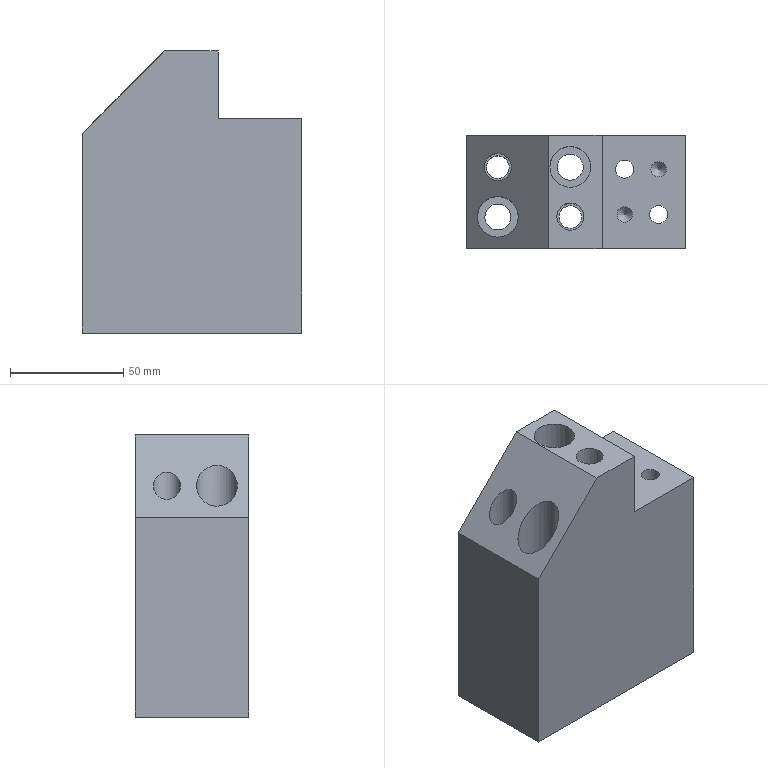Part | NX | features solid 2 | 1 solid | 31 faces | box 97 x 50 x 124.5 mm | volume 427317 mm3 | plane 15 | cylinder 14 | cone 2 | commonest cylinder face diameters 6.8 x2 8.001 x2 10 x2 10.001 x2 11.5 x2 12 x2
STEP:
#1=CARTESIAN_POINT('',(3590.806,-25.,-128.));
#2=VERTEX_POINT('',#1);
#3=CARTESIAN_POINT('',(3590.806,-25.,-39.936));
#4=VERTEX_POINT('',#3);
#5=CARTESIAN_POINT('',(3590.806,-25.,-33.5));
#6=DIRECTION('',(0.,0.,1.));
#7=VECTOR('',#6,1000.);
#8=LINE('',#5,#7);
#9=EDGE_CURVE('',#2,#4,#8,.T.);
#10=ORIENTED_EDGE('',*,*,#9,.T.);
#11=CARTESIAN_POINT('',(3590.806,25.,-39.936));
#12=VERTEX_POINT('',#11);
#13=CARTESIAN_POINT('',(3590.806,0.,-39.936));
#14=DIRECTION('',(0.,1.,0.));
#15=VECTOR('',#14,1000.);
#16=LINE('',#13,#15);
#17=EDGE_CURVE('',#4,#12,#16,.T.);
#18=ORIENTED_EDGE('',*,*,#17,.T.);
#19=CARTESIAN_POINT('',(3590.806,25.,-128.));
#20=VERTEX_POINT('',#19);
#21=CARTESIAN_POINT('',(3590.806,25.,-33.5));
#22=DIRECTION('',(0.,0.,1.));
#23=VECTOR('',#22,1000.);
#24=LINE('',#21,#23);
#25=EDGE_CURVE('',#20,#12,#24,.T.);
#26=ORIENTED_EDGE('',*,*,#25,.F.);
#27=CARTESIAN_POINT('',(3590.806,193.,-128.));
#28=DIRECTION('',(0.,-1.,0.));
#29=VECTOR('',#28,1000.);
#30=LINE('',#27,#29);
#31=EDGE_CURVE('',#20,#2,#30,.T.);
#32=ORIENTED_EDGE('',*,*,#31,.T.);
#33=EDGE_LOOP('',(#10,#18,#26,#32));
#34=FACE_BOUND('',#33,.T.);
#35=CARTESIAN_POINT('',(3590.806,0.,-33.5));
#36=DIRECTION('',(-1.,0.,0.));
#37=DIRECTION('',(0.,0.,-1.));
#38=AXIS2_PLACEMENT_3D('',#35,#36,#37);
#39=PLANE('',#38);
#40=ADVANCED_FACE('',(#34),#39,.T.);
#41=ORIENTED_EDGE('',*,*,#25,.T.);
#42=CARTESIAN_POINT('',(3627.243,25.,-3.5));
#43=VERTEX_POINT('',#42);
#44=CARTESIAN_POINT('',(3614.025,25.,-16.718));
#45=DIRECTION('',(0.7071,0.,0.7071));
#46=VECTOR('',#45,1000.);
#47=LINE('',#44,#46);
#48=EDGE_CURVE('',#12,#43,#47,.T.);
#49=ORIENTED_EDGE('',*,*,#48,.T.);
#50=CARTESIAN_POINT('',(3650.806,25.,-3.5));
#51=VERTEX_POINT('',#50);
#52=CARTESIAN_POINT('',(3630.806,25.,-3.5));
#53=DIRECTION('',(1.,0.,0.));
#54=VECTOR('',#53,1000.);
#55=LINE('',#52,#54);
#56=EDGE_CURVE('',#43,#51,#55,.T.);
#57=ORIENTED_EDGE('',*,*,#56,.T.);
#58=CARTESIAN_POINT('',(3650.806,25.,-33.5));
#59=VERTEX_POINT('',#58);
#60=CARTESIAN_POINT('',(3650.806,25.,-33.5));
#61=DIRECTION('',(0.,0.,1.));
#62=VECTOR('',#61,1000.);
#63=LINE('',#60,#62);
#64=EDGE_CURVE('',#59,#51,#63,.T.);
#65=ORIENTED_EDGE('',*,*,#64,.F.);
#66=CARTESIAN_POINT('',(3687.806,25.,-33.5));
#67=VERTEX_POINT('',#66);
#68=CARTESIAN_POINT('',(3630.806,25.,-33.5));
#69=DIRECTION('',(1.,0.,0.));
#70=VECTOR('',#69,1000.);
#71=LINE('',#68,#70);
#72=EDGE_CURVE('',#59,#67,#71,.T.);
#73=ORIENTED_EDGE('',*,*,#72,.T.);
#74=CARTESIAN_POINT('',(3687.806,25.,-128.));
#75=VERTEX_POINT('',#74);
#76=CARTESIAN_POINT('',(3687.806,25.,-33.5));
#77=DIRECTION('',(0.,0.,1.));
#78=VECTOR('',#77,1000.);
#79=LINE('',#76,#78);
#80=EDGE_CURVE('',#75,#67,#79,.T.);
#81=ORIENTED_EDGE('',*,*,#80,.F.);
#82=CARTESIAN_POINT('',(3630.806,25.,-128.));
#83=DIRECTION('',(1.,0.,0.));
#84=VECTOR('',#83,1000.);
#85=LINE('',#82,#84);
#86=EDGE_CURVE('',#20,#75,#85,.T.);
#87=ORIENTED_EDGE('',*,*,#86,.F.);
#88=EDGE_LOOP('',(#41,#49,#57,#65,#73,#81,#87));
#89=FACE_BOUND('',#88,.T.);
#90=CARTESIAN_POINT('',(3630.806,25.,-33.5));
#91=DIRECTION('',(0.,1.,0.));
#92=DIRECTION('',(0.,0.,-1.));
#93=AXIS2_PLACEMENT_3D('',#90,#91,#92);
#94=PLANE('',#93);
#95=ADVANCED_FACE('',(#89),#94,.T.);
#96=CARTESIAN_POINT('',(3627.243,-25.,-3.5));
#97=VERTEX_POINT('',#96);
#98=CARTESIAN_POINT('',(3614.025,-25.,-16.718));
#99=DIRECTION('',(0.7071,0.,0.7071));
#100=VECTOR('',#99,1000.);
#101=LINE('',#98,#100);
#102=EDGE_CURVE('',#4,#97,#101,.T.);
#103=ORIENTED_EDGE('',*,*,#102,.F.);
#104=ORIENTED_EDGE('',*,*,#9,.F.);
#105=CARTESIAN_POINT('',(3687.806,-25.,-128.));
#106=VERTEX_POINT('',#105);
#107=CARTESIAN_POINT('',(3630.806,-25.,-128.));
#108=DIRECTION('',(1.,0.,0.));
#109=VECTOR('',#108,1000.);
#110=LINE('',#107,#109);
#111=EDGE_CURVE('',#2,#106,#110,.T.);
#112=ORIENTED_EDGE('',*,*,#111,.T.);
#113=CARTESIAN_POINT('',(3687.806,-25.,-33.5));
#114=VERTEX_POINT('',#113);
#115=CARTESIAN_POINT('',(3687.806,-25.,-33.5));
#116=DIRECTION('',(0.,0.,1.));
#117=VECTOR('',#116,1000.);
#118=LINE('',#115,#117);
#119=EDGE_CURVE('',#106,#114,#118,.T.);
#120=ORIENTED_EDGE('',*,*,#119,.T.);
#121=CARTESIAN_POINT('',(3650.806,-25.,-33.5));
#122=VERTEX_POINT('',#121);
#123=CARTESIAN_POINT('',(3630.806,-25.,-33.5));
#124=DIRECTION('',(1.,0.,0.));
#125=VECTOR('',#124,1000.);
#126=LINE('',#123,#125);
#127=EDGE_CURVE('',#122,#114,#126,.T.);
#128=ORIENTED_EDGE('',*,*,#127,.F.);
#129=CARTESIAN_POINT('',(3650.806,-25.,-3.5));
#130=VERTEX_POINT('',#129);
#131=CARTESIAN_POINT('',(3650.806,-25.,-33.5));
#132=DIRECTION('',(0.,0.,1.));
#133=VECTOR('',#132,1000.);
#134=LINE('',#131,#133);
#135=EDGE_CURVE('',#122,#130,#134,.T.);
#136=ORIENTED_EDGE('',*,*,#135,.T.);
#137=CARTESIAN_POINT('',(3630.806,-25.,-3.5));
#138=DIRECTION('',(1.,0.,0.));
#139=VECTOR('',#138,1000.);
#140=LINE('',#137,#139);
#141=EDGE_CURVE('',#97,#130,#140,.T.);
#142=ORIENTED_EDGE('',*,*,#141,.F.);
#143=EDGE_LOOP('',(#103,#104,#112,#120,#128,#136,#142));
#144=FACE_BOUND('',#143,.T.);
#145=CARTESIAN_POINT('',(3630.806,-25.,-33.5));
#146=DIRECTION('',(0.,1.,0.));
#147=DIRECTION('',(0.,0.,-1.));
#148=AXIS2_PLACEMENT_3D('',#145,#146,#147);
#149=PLANE('',#148);
#150=ADVANCED_FACE('',(#144),#149,.F.);
#151=CARTESIAN_POINT('',(3630.806,-11.,-3.5));
#152=VERTEX_POINT('',#151);
#153=CARTESIAN_POINT('',(3636.806,-11.,-3.5));
#154=DIRECTION('',(0.,0.,-1.));
#155=DIRECTION('',(-1.,0.,0.));
#156=AXIS2_PLACEMENT_3D('',#153,#154,#155);
#157=CIRCLE('',#156,6.);
#158=EDGE_CURVE('',#152,#152,#157,.T.);
#159=ORIENTED_EDGE('',*,*,#158,.T.);
#160=EDGE_LOOP('',(#159));
#161=FACE_BOUND('',#160,.T.);
#162=CARTESIAN_POINT('',(3645.806,11.,-3.5));
#163=VERTEX_POINT('',#162);
#164=CARTESIAN_POINT('',(3636.806,11.,-3.5));
#165=DIRECTION('',(0.,0.,-1.));
#166=DIRECTION('',(1.,0.,0.));
#167=AXIS2_PLACEMENT_3D('',#164,#165,#166);
#168=CIRCLE('',#167,9.);
#169=EDGE_CURVE('',#163,#163,#168,.T.);
#170=ORIENTED_EDGE('',*,*,#169,.T.);
#171=EDGE_LOOP('',(#170));
#172=FACE_BOUND('',#171,.T.);
#173=CARTESIAN_POINT('',(3627.243,0.,-3.5));
#174=DIRECTION('',(0.,1.,0.));
#175=VECTOR('',#174,1000.);
#176=LINE('',#173,#175);
#177=EDGE_CURVE('',#97,#43,#176,.T.);
#178=ORIENTED_EDGE('',*,*,#177,.F.);
#179=ORIENTED_EDGE('',*,*,#141,.T.);
#180=CARTESIAN_POINT('',(3650.806,0.,-3.5));
#181=DIRECTION('',(0.,1.,0.));
#182=VECTOR('',#181,1000.);
#183=LINE('',#180,#182);
#184=EDGE_CURVE('',#130,#51,#183,.T.);
#185=ORIENTED_EDGE('',*,*,#184,.T.);
#186=ORIENTED_EDGE('',*,*,#56,.F.);
#187=EDGE_LOOP('',(#178,#179,#185,#186));
#188=FACE_BOUND('',#187,.T.);
#189=CARTESIAN_POINT('',(3630.806,0.,-3.5));
#190=DIRECTION('',(0.,0.,-1.));
#191=DIRECTION('',(1.,0.,0.));
#192=AXIS2_PLACEMENT_3D('',#189,#190,#191);
#193=PLANE('',#192);
#194=ADVANCED_FACE('',(#161,#172,#188),#193,.F.);
#195=CARTESIAN_POINT('',(3610.806,11.,-102.));
#196=VERTEX_POINT('',#195);
#197=CARTESIAN_POINT('',(3604.806,11.,-102.));
#198=DIRECTION('',(0.,0.,-1.));
#199=DIRECTION('',(1.,0.,0.));
#200=AXIS2_PLACEMENT_3D('',#197,#198,#199);
#201=CIRCLE('',#200,6.);
#202=EDGE_CURVE('',#196,#196,#201,.T.);
#203=ORIENTED_EDGE('',*,*,#202,.T.);
#204=EDGE_LOOP('',(#203));
#205=FACE_BOUND('',#204,.T.);
#206=CARTESIAN_POINT('',(3598.806,11.,-31.936));
#207=VERTEX_POINT('',#206);
#208=CARTESIAN_POINT('',(3604.806,11.,-25.936));
#209=DIRECTION('',(0.7071,0.,-0.7071));
#210=DIRECTION('',(-0.7071,0.,-0.7071));
#211=AXIS2_PLACEMENT_3D('',#208,#209,#210);
#212=ELLIPSE('',#211,8.485,6.);
#213=EDGE_CURVE('',#207,#207,#212,.T.);
#214=ORIENTED_EDGE('',*,*,#213,.F.);
#215=EDGE_LOOP('',(#214));
#216=FACE_BOUND('',#215,.T.);
#217=CARTESIAN_POINT('',(3604.806,11.,-1.5));
#218=DIRECTION('',(0.,0.,-1.));
#219=DIRECTION('',(-1.,0.,0.));
#220=AXIS2_PLACEMENT_3D('',#217,#218,#219);
#221=CYLINDRICAL_SURFACE('',#220,6.);
#222=ADVANCED_FACE('',(#205,#216),#221,.F.);
#223=CARTESIAN_POINT('',(3613.806,-11.,-98.));
#224=VERTEX_POINT('',#223);
#225=CARTESIAN_POINT('',(3604.806,-11.,-98.));
#226=DIRECTION('',(0.,0.,-1.));
#227=DIRECTION('',(1.,0.,0.));
#228=AXIS2_PLACEMENT_3D('',#225,#226,#227);
#229=CIRCLE('',#228,9.);
#230=EDGE_CURVE('',#224,#224,#229,.T.);
#231=ORIENTED_EDGE('',*,*,#230,.T.);
#232=EDGE_LOOP('',(#231));
#233=FACE_BOUND('',#232,.T.);
#234=CARTESIAN_POINT('',(3595.806,-11.,-34.936));
#235=VERTEX_POINT('',#234);
#236=CARTESIAN_POINT('',(3604.806,-11.,-25.936));
#237=DIRECTION('',(0.7071,0.,-0.7071));
#238=DIRECTION('',(-0.7071,0.,-0.7071));
#239=AXIS2_PLACEMENT_3D('',#236,#237,#238);
#240=ELLIPSE('',#239,12.728,9.);
#241=EDGE_CURVE('',#235,#235,#240,.T.);
#242=ORIENTED_EDGE('',*,*,#241,.F.);
#243=EDGE_LOOP('',(#242));
#244=FACE_BOUND('',#243,.T.);
#245=CARTESIAN_POINT('',(3604.806,-11.,-3.5));
#246=DIRECTION('',(0.,0.,-1.));
#247=DIRECTION('',(-1.,0.,0.));
#248=AXIS2_PLACEMENT_3D('',#245,#246,#247);
#249=CYLINDRICAL_SURFACE('',#248,9.);
#250=ADVANCED_FACE('',(#233,#244),#249,.F.);
#251=CARTESIAN_POINT('',(3679.206,10.,-33.5));
#252=VERTEX_POINT('',#251);
#253=CARTESIAN_POINT('',(3675.806,10.,-33.5));
#254=DIRECTION('',(0.,0.,-1.));
#255=DIRECTION('',(1.,0.,0.));
#256=AXIS2_PLACEMENT_3D('',#253,#254,#255);
#257=CIRCLE('',#256,3.4);
#258=EDGE_CURVE('',#252,#252,#257,.T.);
#259=ORIENTED_EDGE('',*,*,#258,.T.);
#260=EDGE_LOOP('',(#259));
#261=FACE_BOUND('',#260,.T.);
#262=CARTESIAN_POINT('',(3664.807,10.,-33.5));
#263=VERTEX_POINT('',#262);
#264=CARTESIAN_POINT('',(3660.806,10.,-33.5));
#265=DIRECTION('',(0.,0.,-1.));
#266=DIRECTION('',(1.,0.,0.));
#267=AXIS2_PLACEMENT_3D('',#264,#265,#266);
#268=CIRCLE('',#267,4.);
#269=EDGE_CURVE('',#263,#263,#268,.T.);
#270=ORIENTED_EDGE('',*,*,#269,.T.);
#271=EDGE_LOOP('',(#270));
#272=FACE_BOUND('',#271,.T.);
#273=CARTESIAN_POINT('',(3679.807,-10.,-33.5));
#274=VERTEX_POINT('',#273);
#275=CARTESIAN_POINT('',(3675.806,-10.,-33.5));
#276=DIRECTION('',(0.,0.,-1.));
#277=DIRECTION('',(1.,0.,0.));
#278=AXIS2_PLACEMENT_3D('',#275,#276,#277);
#279=CIRCLE('',#278,4.);
#280=EDGE_CURVE('',#274,#274,#279,.T.);
#281=ORIENTED_EDGE('',*,*,#280,.T.);
#282=EDGE_LOOP('',(#281));
#283=FACE_BOUND('',#282,.T.);
#284=CARTESIAN_POINT('',(3664.206,-10.,-33.5));
#285=VERTEX_POINT('',#284);
#286=CARTESIAN_POINT('',(3660.806,-10.,-33.5));
#287=DIRECTION('',(0.,0.,-1.));
#288=DIRECTION('',(1.,0.,0.));
#289=AXIS2_PLACEMENT_3D('',#286,#287,#288);
#290=CIRCLE('',#289,3.4);
#291=EDGE_CURVE('',#285,#285,#290,.T.);
#292=ORIENTED_EDGE('',*,*,#291,.T.);
#293=EDGE_LOOP('',(#292));
#294=FACE_BOUND('',#293,.T.);
#295=CARTESIAN_POINT('',(3650.806,0.,-33.5));
#296=DIRECTION('',(0.,1.,0.));
#297=VECTOR('',#296,1000.);
#298=LINE('',#295,#297);
#299=EDGE_CURVE('',#122,#59,#298,.T.);
#300=ORIENTED_EDGE('',*,*,#299,.F.);
#301=ORIENTED_EDGE('',*,*,#127,.T.);
#302=CARTESIAN_POINT('',(3687.806,0.,-33.5));
#303=DIRECTION('',(0.,-1.,0.));
#304=VECTOR('',#303,1000.);
#305=LINE('',#302,#304);
#306=EDGE_CURVE('',#67,#114,#305,.T.);
#307=ORIENTED_EDGE('',*,*,#306,.F.);
#308=ORIENTED_EDGE('',*,*,#72,.F.);
#309=EDGE_LOOP('',(#300,#301,#307,#308));
#310=FACE_BOUND('',#309,.T.);
#311=CARTESIAN_POINT('',(3675.806,0.,-33.5));
#312=DIRECTION('',(0.,0.,-1.));
#313=DIRECTION('',(1.,0.,0.));
#314=AXIS2_PLACEMENT_3D('',#311,#312,#313);
#315=PLANE('',#314);
#316=ADVANCED_FACE('',(#261,#272,#283,#294,#310),#315,.F.);
#317=CARTESIAN_POINT('',(3655.806,10.,-128.));
#318=VERTEX_POINT('',#317);
#319=CARTESIAN_POINT('',(3660.806,10.,-128.));
#320=DIRECTION('',(0.,0.,1.));
#321=DIRECTION('',(-1.,0.,0.));
#322=AXIS2_PLACEMENT_3D('',#319,#320,#321);
#323=CIRCLE('',#322,5.);
#324=EDGE_CURVE('',#318,#318,#323,.T.);
#325=ORIENTED_EDGE('',*,*,#324,.T.);
#326=EDGE_LOOP('',(#325));
#327=FACE_BOUND('',#326,.T.);
#328=CARTESIAN_POINT('',(3670.806,-10.,-128.));
#329=VERTEX_POINT('',#328);
#330=CARTESIAN_POINT('',(3675.806,-10.,-128.));
#331=DIRECTION('',(0.,0.,1.));
#332=DIRECTION('',(-1.,0.,0.));
#333=AXIS2_PLACEMENT_3D('',#330,#331,#332);
#334=CIRCLE('',#333,5.);
#335=EDGE_CURVE('',#329,#329,#334,.T.);
#336=ORIENTED_EDGE('',*,*,#335,.T.);
#337=EDGE_LOOP('',(#336));
#338=FACE_BOUND('',#337,.T.);
#339=CARTESIAN_POINT('',(3599.056,-11.,-128.));
#340=VERTEX_POINT('',#339);
#341=CARTESIAN_POINT('',(3604.806,-11.,-128.));
#342=DIRECTION('',(0.,0.,1.));
#343=DIRECTION('',(-1.,0.,0.));
#344=AXIS2_PLACEMENT_3D('',#341,#342,#343);
#345=CIRCLE('',#344,5.75);
#346=EDGE_CURVE('',#340,#340,#345,.T.);
#347=ORIENTED_EDGE('',*,*,#346,.T.);
#348=EDGE_LOOP('',(#347));
#349=FACE_BOUND('',#348,.T.);
#350=CARTESIAN_POINT('',(3599.806,11.,-128.));
#351=VERTEX_POINT('',#350);
#352=CARTESIAN_POINT('',(3604.806,11.,-128.));
#353=DIRECTION('',(0.,0.,1.));
#354=DIRECTION('',(-1.,0.,0.));
#355=AXIS2_PLACEMENT_3D('',#352,#353,#354);
#356=CIRCLE('',#355,5.);
#357=EDGE_CURVE('',#351,#351,#356,.T.);
#358=ORIENTED_EDGE('',*,*,#357,.T.);
#359=EDGE_LOOP('',(#358));
#360=FACE_BOUND('',#359,.T.);
#361=CARTESIAN_POINT('',(3631.056,11.,-128.));
#362=VERTEX_POINT('',#361);
#363=CARTESIAN_POINT('',(3636.806,11.,-128.));
#364=DIRECTION('',(0.,0.,1.));
#365=DIRECTION('',(-1.,0.,0.));
#366=AXIS2_PLACEMENT_3D('',#363,#364,#365);
#367=CIRCLE('',#366,5.75);
#368=EDGE_CURVE('',#362,#362,#367,.T.);
#369=ORIENTED_EDGE('',*,*,#368,.T.);
#370=EDGE_LOOP('',(#369));
#371=FACE_BOUND('',#370,.T.);
#372=CARTESIAN_POINT('',(3631.806,-11.,-128.));
#373=VERTEX_POINT('',#372);
#374=CARTESIAN_POINT('',(3636.806,-11.,-128.));
#375=DIRECTION('',(0.,0.,1.));
#376=DIRECTION('',(-1.,0.,0.));
#377=AXIS2_PLACEMENT_3D('',#374,#375,#376);
#378=CIRCLE('',#377,5.);
#379=EDGE_CURVE('',#373,#373,#378,.T.);
#380=ORIENTED_EDGE('',*,*,#379,.T.);
#381=EDGE_LOOP('',(#380));
#382=FACE_BOUND('',#381,.T.);
#383=CARTESIAN_POINT('',(3687.806,193.,-128.));
#384=DIRECTION('',(0.,-1.,0.));
#385=VECTOR('',#384,1000.);
#386=LINE('',#383,#385);
#387=EDGE_CURVE('',#75,#106,#386,.T.);
#388=ORIENTED_EDGE('',*,*,#387,.T.);
#389=ORIENTED_EDGE('',*,*,#111,.F.);
#390=ORIENTED_EDGE('',*,*,#31,.F.);
#391=ORIENTED_EDGE('',*,*,#86,.T.);
#392=EDGE_LOOP('',(#388,#389,#390,#391));
#393=FACE_BOUND('',#392,.T.);
#394=CARTESIAN_POINT('',(282.5,193.,-128.));
#395=DIRECTION('',(0.,0.,-1.));
#396=DIRECTION('',(-1.,0.,0.));
#397=AXIS2_PLACEMENT_3D('',#394,#395,#396);
#398=PLANE('',#397);
#399=ADVANCED_FACE('',(#327,#338,#349,#360,#371,#382,#393),#398,.T.);
#400=ORIENTED_EDGE('',*,*,#80,.T.);
#401=ORIENTED_EDGE('',*,*,#306,.T.);
#402=ORIENTED_EDGE('',*,*,#119,.F.);
#403=ORIENTED_EDGE('',*,*,#387,.F.);
#404=EDGE_LOOP('',(#400,#401,#402,#403));
#405=FACE_BOUND('',#404,.T.);
#406=CARTESIAN_POINT('',(3687.806,0.,-33.5));
#407=DIRECTION('',(1.,0.,0.));
#408=DIRECTION('',(0.,0.,1.));
#409=AXIS2_PLACEMENT_3D('',#406,#407,#408);
#410=PLANE('',#409);
#411=ADVANCED_FACE('',(#405),#410,.T.);
#412=ORIENTED_EDGE('',*,*,#299,.T.);
#413=ORIENTED_EDGE('',*,*,#64,.T.);
#414=ORIENTED_EDGE('',*,*,#184,.F.);
#415=ORIENTED_EDGE('',*,*,#135,.F.);
#416=EDGE_LOOP('',(#412,#413,#414,#415));
#417=FACE_BOUND('',#416,.T.);
#418=CARTESIAN_POINT('',(3650.806,0.,-33.5));
#419=DIRECTION('',(-1.,0.,0.));
#420=DIRECTION('',(0.,0.,-1.));
#421=AXIS2_PLACEMENT_3D('',#418,#419,#420);
#422=PLANE('',#421);
#423=ADVANCED_FACE('',(#417),#422,.F.);
#424=CARTESIAN_POINT('',(3631.806,-11.,-102.));
#425=VERTEX_POINT('',#424);
#426=CARTESIAN_POINT('',(3636.806,-11.,-102.));
#427=DIRECTION('',(0.,0.,-1.));
#428=DIRECTION('',(-1.,0.,0.));
#429=AXIS2_PLACEMENT_3D('',#426,#427,#428);
#430=CIRCLE('',#429,5.);
#431=EDGE_CURVE('',#425,#425,#430,.T.);
#432=ORIENTED_EDGE('',*,*,#431,.F.);
#433=EDGE_LOOP('',(#432));
#434=FACE_BOUND('',#433,.T.);
#435=ORIENTED_EDGE('',*,*,#379,.F.);
#436=EDGE_LOOP('',(#435));
#437=FACE_BOUND('',#436,.T.);
#438=CARTESIAN_POINT('',(3636.806,-11.,-1.5));
#439=DIRECTION('',(0.,0.,-1.));
#440=DIRECTION('',(-1.,0.,0.));
#441=AXIS2_PLACEMENT_3D('',#438,#439,#440);
#442=CYLINDRICAL_SURFACE('',#441,5.);
#443=ADVANCED_FACE('',(#434,#437),#442,.F.);
#444=CARTESIAN_POINT('',(3642.806,-11.,-102.));
#445=VERTEX_POINT('',#444);
#446=CARTESIAN_POINT('',(3636.806,-11.,-102.));
#447=DIRECTION('',(0.,0.,-1.));
#448=DIRECTION('',(1.,0.,0.));
#449=AXIS2_PLACEMENT_3D('',#446,#447,#448);
#450=CIRCLE('',#449,6.);
#451=EDGE_CURVE('',#445,#445,#450,.T.);
#452=ORIENTED_EDGE('',*,*,#451,.T.);
#453=EDGE_LOOP('',(#452));
#454=FACE_BOUND('',#453,.T.);
#455=ORIENTED_EDGE('',*,*,#158,.F.);
#456=EDGE_LOOP('',(#455));
#457=FACE_BOUND('',#456,.T.);
#458=CARTESIAN_POINT('',(3636.806,-11.,-1.5));
#459=DIRECTION('',(0.,0.,-1.));
#460=DIRECTION('',(-1.,0.,0.));
#461=AXIS2_PLACEMENT_3D('',#458,#459,#460);
#462=CYLINDRICAL_SURFACE('',#461,6.);
#463=ADVANCED_FACE('',(#454,#457),#462,.F.);
#464=ORIENTED_EDGE('',*,*,#431,.T.);
#465=EDGE_LOOP('',(#464));
#466=FACE_BOUND('',#465,.T.);
#467=ORIENTED_EDGE('',*,*,#451,.F.);
#468=EDGE_LOOP('',(#467));
#469=FACE_BOUND('',#468,.T.);
#470=CARTESIAN_POINT('',(3636.806,-11.,-102.));
#471=DIRECTION('',(0.,0.,-1.));
#472=DIRECTION('',(1.,0.,0.));
#473=AXIS2_PLACEMENT_3D('',#470,#471,#472);
#474=PLANE('',#473);
#475=ADVANCED_FACE('',(#466,#469),#474,.F.);
#476=CARTESIAN_POINT('',(3631.056,11.,-98.));
#477=VERTEX_POINT('',#476);
#478=CARTESIAN_POINT('',(3636.806,11.,-98.));
#479=DIRECTION('',(0.,0.,-1.));
#480=DIRECTION('',(-1.,0.,0.));
#481=AXIS2_PLACEMENT_3D('',#478,#479,#480);
#482=CIRCLE('',#481,5.75);
#483=EDGE_CURVE('',#477,#477,#482,.T.);
#484=ORIENTED_EDGE('',*,*,#483,.F.);
#485=EDGE_LOOP('',(#484));
#486=FACE_BOUND('',#485,.T.);
#487=ORIENTED_EDGE('',*,*,#368,.F.);
#488=EDGE_LOOP('',(#487));
#489=FACE_BOUND('',#488,.T.);
#490=CARTESIAN_POINT('',(3636.806,11.,-1.5));
#491=DIRECTION('',(0.,0.,-1.));
#492=DIRECTION('',(-1.,0.,0.));
#493=AXIS2_PLACEMENT_3D('',#490,#491,#492);
#494=CYLINDRICAL_SURFACE('',#493,5.75);
#495=ADVANCED_FACE('',(#486,#489),#494,.F.);
#496=ORIENTED_EDGE('',*,*,#483,.T.);
#497=EDGE_LOOP('',(#496));
#498=FACE_BOUND('',#497,.T.);
#499=CARTESIAN_POINT('',(3645.806,11.,-98.));
#500=VERTEX_POINT('',#499);
#501=CARTESIAN_POINT('',(3636.806,11.,-98.));
#502=DIRECTION('',(0.,0.,-1.));
#503=DIRECTION('',(1.,0.,0.));
#504=AXIS2_PLACEMENT_3D('',#501,#502,#503);
#505=CIRCLE('',#504,9.);
#506=EDGE_CURVE('',#500,#500,#505,.T.);
#507=ORIENTED_EDGE('',*,*,#506,.F.);
#508=EDGE_LOOP('',(#507));
#509=FACE_BOUND('',#508,.T.);
#510=CARTESIAN_POINT('',(3636.806,11.,-98.));
#511=DIRECTION('',(0.,0.,-1.));
#512=DIRECTION('',(1.,0.,0.));
#513=AXIS2_PLACEMENT_3D('',#510,#511,#512);
#514=PLANE('',#513);
#515=ADVANCED_FACE('',(#498,#509),#514,.F.);
#516=ORIENTED_EDGE('',*,*,#506,.T.);
#517=EDGE_LOOP('',(#516));
#518=FACE_BOUND('',#517,.T.);
#519=ORIENTED_EDGE('',*,*,#169,.F.);
#520=EDGE_LOOP('',(#519));
#521=FACE_BOUND('',#520,.T.);
#522=CARTESIAN_POINT('',(3636.806,11.,-3.5));
#523=DIRECTION('',(0.,0.,-1.));
#524=DIRECTION('',(-1.,0.,0.));
#525=AXIS2_PLACEMENT_3D('',#522,#523,#524);
#526=CYLINDRICAL_SURFACE('',#525,9.);
#527=ADVANCED_FACE('',(#518,#521),#526,.F.);
#528=CARTESIAN_POINT('',(3599.806,11.,-102.));
#529=VERTEX_POINT('',#528);
#530=CARTESIAN_POINT('',(3604.806,11.,-102.));
#531=DIRECTION('',(0.,0.,-1.));
#532=DIRECTION('',(-1.,0.,0.));
#533=AXIS2_PLACEMENT_3D('',#530,#531,#532);
#534=CIRCLE('',#533,5.);
#535=EDGE_CURVE('',#529,#529,#534,.T.);
#536=ORIENTED_EDGE('',*,*,#535,.F.);
#537=EDGE_LOOP('',(#536));
#538=FACE_BOUND('',#537,.T.);
#539=ORIENTED_EDGE('',*,*,#357,.F.);
#540=EDGE_LOOP('',(#539));
#541=FACE_BOUND('',#540,.T.);
#542=CARTESIAN_POINT('',(3604.806,11.,-1.5));
#543=DIRECTION('',(0.,0.,-1.));
#544=DIRECTION('',(-1.,0.,0.));
#545=AXIS2_PLACEMENT_3D('',#542,#543,#544);
#546=CYLINDRICAL_SURFACE('',#545,5.);
#547=ADVANCED_FACE('',(#538,#541),#546,.F.);
#548=ORIENTED_EDGE('',*,*,#535,.T.);
#549=EDGE_LOOP('',(#548));
#550=FACE_BOUND('',#549,.T.);
#551=ORIENTED_EDGE('',*,*,#202,.F.);
#552=EDGE_LOOP('',(#551));
#553=FACE_BOUND('',#552,.T.);
#554=CARTESIAN_POINT('',(3604.806,11.,-102.));
#555=DIRECTION('',(0.,0.,-1.));
#556=DIRECTION('',(1.,0.,0.));
#557=AXIS2_PLACEMENT_3D('',#554,#555,#556);
#558=PLANE('',#557);
#559=ADVANCED_FACE('',(#550,#553),#558,.F.);
#560=CARTESIAN_POINT('',(3599.056,-11.,-98.));
#561=VERTEX_POINT('',#560);
#562=CARTESIAN_POINT('',(3604.806,-11.,-98.));
#563=DIRECTION('',(0.,0.,-1.));
#564=DIRECTION('',(-1.,0.,0.));
#565=AXIS2_PLACEMENT_3D('',#562,#563,#564);
#566=CIRCLE('',#565,5.75);
#567=EDGE_CURVE('',#561,#561,#566,.T.);
#568=ORIENTED_EDGE('',*,*,#567,.F.);
#569=EDGE_LOOP('',(#568));
#570=FACE_BOUND('',#569,.T.);
#571=ORIENTED_EDGE('',*,*,#346,.F.);
#572=EDGE_LOOP('',(#571));
#573=FACE_BOUND('',#572,.T.);
#574=CARTESIAN_POINT('',(3604.806,-11.,-1.5));
#575=DIRECTION('',(0.,0.,-1.));
#576=DIRECTION('',(-1.,0.,0.));
#577=AXIS2_PLACEMENT_3D('',#574,#575,#576);
#578=CYLINDRICAL_SURFACE('',#577,5.75);
#579=ADVANCED_FACE('',(#570,#573),#578,.F.);
#580=ORIENTED_EDGE('',*,*,#567,.T.);
#581=EDGE_LOOP('',(#580));
#582=FACE_BOUND('',#581,.T.);
#583=ORIENTED_EDGE('',*,*,#230,.F.);
#584=EDGE_LOOP('',(#583));
#585=FACE_BOUND('',#584,.T.);
#586=CARTESIAN_POINT('',(3604.806,-11.,-98.));
#587=DIRECTION('',(0.,0.,-1.));
#588=DIRECTION('',(1.,0.,0.));
#589=AXIS2_PLACEMENT_3D('',#586,#587,#588);
#590=PLANE('',#589);
#591=ADVANCED_FACE('',(#582,#585),#590,.F.);
#592=ORIENTED_EDGE('',*,*,#17,.F.);
#593=ORIENTED_EDGE('',*,*,#102,.T.);
#594=ORIENTED_EDGE('',*,*,#177,.T.);
#595=ORIENTED_EDGE('',*,*,#48,.F.);
#596=EDGE_LOOP('',(#592,#593,#594,#595));
#597=FACE_BOUND('',#596,.T.);
#598=ORIENTED_EDGE('',*,*,#241,.T.);
#599=EDGE_LOOP('',(#598));
#600=FACE_BOUND('',#599,.T.);
#601=ORIENTED_EDGE('',*,*,#213,.T.);
#602=EDGE_LOOP('',(#601));
#603=FACE_BOUND('',#602,.T.);
#604=CARTESIAN_POINT('',(3605.121,0.,-25.621));
#605=DIRECTION('',(-0.7071,0.,0.7071));
#606=DIRECTION('',(-0.7071,0.,-0.7071));
#607=AXIS2_PLACEMENT_3D('',#604,#605,#606);
#608=PLANE('',#607);
#609=ADVANCED_FACE('',(#597,#600,#603),#608,.T.);
#610=CARTESIAN_POINT('',(3657.406,-10.,-59.1));
#611=VERTEX_POINT('',#610);
#612=CARTESIAN_POINT('',(3660.806,-10.,-59.1));
#613=DIRECTION('',(0.,0.,-1.));
#614=DIRECTION('',(-1.,0.,0.));
#615=AXIS2_PLACEMENT_3D('',#612,#613,#614);
#616=CIRCLE('',#615,3.4);
#617=EDGE_CURVE('',#611,#611,#616,.T.);
#618=ORIENTED_EDGE('',*,*,#617,.T.);
#619=EDGE_LOOP('',(#618));
#620=FACE_BOUND('',#619,.T.);
#621=ORIENTED_EDGE('',*,*,#291,.F.);
#622=EDGE_LOOP('',(#621));
#623=FACE_BOUND('',#622,.T.);
#624=CARTESIAN_POINT('',(3660.806,-10.,-33.5));
#625=DIRECTION('',(0.,0.,-1.));
#626=DIRECTION('',(-1.,0.,0.));
#627=AXIS2_PLACEMENT_3D('',#624,#625,#626);
#628=CYLINDRICAL_SURFACE('',#627,3.4);
#629=ADVANCED_FACE('',(#620,#623),#628,.F.);
#630=CARTESIAN_POINT('',(3660.806,-10.,-62.5));
#631=VERTEX_POINT('',#630);
#632=VERTEX_LOOP('',#631);
#633=FACE_BOUND('',#632,.T.);
#634=ORIENTED_EDGE('',*,*,#617,.F.);
#635=EDGE_LOOP('',(#634));
#636=FACE_BOUND('',#635,.T.);
#637=CARTESIAN_POINT('',(3660.806,-10.,-59.1));
#638=DIRECTION('',(0.,0.,1.));
#639=DIRECTION('',(-1.,0.,0.));
#640=AXIS2_PLACEMENT_3D('',#637,#638,#639);
#641=CONICAL_SURFACE('',#640,3.4,0.7854);
#642=ADVANCED_FACE('',(#633,#636),#641,.F.);
#643=CARTESIAN_POINT('',(3680.806,-10.,-58.5));
#644=VERTEX_POINT('',#643);
#645=CARTESIAN_POINT('',(3675.806,-10.,-58.5));
#646=DIRECTION('',(0.,0.,1.));
#647=DIRECTION('',(1.,0.,0.));
#648=AXIS2_PLACEMENT_3D('',#645,#646,#647);
#649=CIRCLE('',#648,5.);
#650=EDGE_CURVE('',#644,#644,#649,.T.);
#651=ORIENTED_EDGE('',*,*,#650,.T.);
#652=EDGE_LOOP('',(#651));
#653=FACE_BOUND('',#652,.T.);
#654=ORIENTED_EDGE('',*,*,#335,.F.);
#655=EDGE_LOOP('',(#654));
#656=FACE_BOUND('',#655,.T.);
#657=CARTESIAN_POINT('',(3675.806,-10.,-58.5));
#658=DIRECTION('',(0.,0.,-1.));
#659=DIRECTION('',(-1.,0.,0.));
#660=AXIS2_PLACEMENT_3D('',#657,#658,#659);
#661=CYLINDRICAL_SURFACE('',#660,5.);
#662=ADVANCED_FACE('',(#653,#656),#661,.F.);
#663=CARTESIAN_POINT('',(3679.807,-10.,-58.5));
#664=VERTEX_POINT('',#663);
#665=CARTESIAN_POINT('',(3675.806,-10.,-58.5));
#666=DIRECTION('',(0.,0.,-1.));
#667=DIRECTION('',(1.,0.,0.));
#668=AXIS2_PLACEMENT_3D('',#665,#666,#667);
#669=CIRCLE('',#668,4.);
#670=EDGE_CURVE('',#664,#664,#669,.T.);
#671=ORIENTED_EDGE('',*,*,#670,.F.);
#672=EDGE_LOOP('',(#671));
#673=FACE_BOUND('',#672,.T.);
#674=ORIENTED_EDGE('',*,*,#650,.F.);
#675=EDGE_LOOP('',(#674));
#676=FACE_BOUND('',#675,.T.);
#677=CARTESIAN_POINT('',(3675.806,-10.,-58.5));
#678=DIRECTION('',(0.,0.,1.));
#679=DIRECTION('',(-1.,0.,0.));
#680=AXIS2_PLACEMENT_3D('',#677,#678,#679);
#681=PLANE('',#680);
#682=ADVANCED_FACE('',(#673,#676),#681,.F.);
#683=ORIENTED_EDGE('',*,*,#670,.T.);
#684=EDGE_LOOP('',(#683));
#685=FACE_BOUND('',#684,.T.);
#686=ORIENTED_EDGE('',*,*,#280,.F.);
#687=EDGE_LOOP('',(#686));
#688=FACE_BOUND('',#687,.T.);
#689=CARTESIAN_POINT('',(3675.806,-10.,-33.5));
#690=DIRECTION('',(0.,0.,-1.));
#691=DIRECTION('',(-1.,0.,0.));
#692=AXIS2_PLACEMENT_3D('',#689,#690,#691);
#693=CYLINDRICAL_SURFACE('',#692,4.);
#694=ADVANCED_FACE('',(#685,#688),#693,.F.);
#695=CARTESIAN_POINT('',(3665.806,10.,-58.5));
#696=VERTEX_POINT('',#695);
#697=CARTESIAN_POINT('',(3660.806,10.,-58.5));
#698=DIRECTION('',(0.,0.,1.));
#699=DIRECTION('',(1.,0.,0.));
#700=AXIS2_PLACEMENT_3D('',#697,#698,#699);
#701=CIRCLE('',#700,5.);
#702=EDGE_CURVE('',#696,#696,#701,.T.);
#703=ORIENTED_EDGE('',*,*,#702,.T.);
#704=EDGE_LOOP('',(#703));
#705=FACE_BOUND('',#704,.T.);
#706=ORIENTED_EDGE('',*,*,#324,.F.);
#707=EDGE_LOOP('',(#706));
#708=FACE_BOUND('',#707,.T.);
#709=CARTESIAN_POINT('',(3660.806,10.,-58.5));
#710=DIRECTION('',(0.,0.,-1.));
#711=DIRECTION('',(-1.,0.,0.));
#712=AXIS2_PLACEMENT_3D('',#709,#710,#711);
#713=CYLINDRICAL_SURFACE('',#712,5.);
#714=ADVANCED_FACE('',(#705,#708),#713,.F.);
#715=CARTESIAN_POINT('',(3664.807,10.,-58.5));
#716=VERTEX_POINT('',#715);
#717=CARTESIAN_POINT('',(3660.806,10.,-58.5));
#718=DIRECTION('',(0.,0.,-1.));
#719=DIRECTION('',(1.,0.,0.));
#720=AXIS2_PLACEMENT_3D('',#717,#718,#719);
#721=CIRCLE('',#720,4.);
#722=EDGE_CURVE('',#716,#716,#721,.T.);
#723=ORIENTED_EDGE('',*,*,#722,.F.);
#724=EDGE_LOOP('',(#723));
#725=FACE_BOUND('',#724,.T.);
#726=ORIENTED_EDGE('',*,*,#702,.F.);
#727=EDGE_LOOP('',(#726));
#728=FACE_BOUND('',#727,.T.);
#729=CARTESIAN_POINT('',(3660.806,10.,-58.5));
#730=DIRECTION('',(0.,0.,1.));
#731=DIRECTION('',(-1.,0.,0.));
#732=AXIS2_PLACEMENT_3D('',#729,#730,#731);
#733=PLANE('',#732);
#734=ADVANCED_FACE('',(#725,#728),#733,.F.);
#735=ORIENTED_EDGE('',*,*,#722,.T.);
#736=EDGE_LOOP('',(#735));
#737=FACE_BOUND('',#736,.T.);
#738=ORIENTED_EDGE('',*,*,#269,.F.);
#739=EDGE_LOOP('',(#738));
#740=FACE_BOUND('',#739,.T.);
#741=CARTESIAN_POINT('',(3660.806,10.,-33.5));
#742=DIRECTION('',(0.,0.,-1.));
#743=DIRECTION('',(-1.,0.,0.));
#744=AXIS2_PLACEMENT_3D('',#741,#742,#743);
#745=CYLINDRICAL_SURFACE('',#744,4.);
#746=ADVANCED_FACE('',(#737,#740),#745,.F.);
#747=CARTESIAN_POINT('',(3672.406,10.,-59.1));
#748=VERTEX_POINT('',#747);
#749=CARTESIAN_POINT('',(3675.806,10.,-59.1));
#750=DIRECTION('',(0.,0.,-1.));
#751=DIRECTION('',(-1.,0.,0.));
#752=AXIS2_PLACEMENT_3D('',#749,#750,#751);
#753=CIRCLE('',#752,3.4);
#754=EDGE_CURVE('',#748,#748,#753,.T.);
#755=ORIENTED_EDGE('',*,*,#754,.T.);
#756=EDGE_LOOP('',(#755));
#757=FACE_BOUND('',#756,.T.);
#758=ORIENTED_EDGE('',*,*,#258,.F.);
#759=EDGE_LOOP('',(#758));
#760=FACE_BOUND('',#759,.T.);
#761=CARTESIAN_POINT('',(3675.806,10.,-33.5));
#762=DIRECTION('',(0.,0.,-1.));
#763=DIRECTION('',(-1.,0.,0.));
#764=AXIS2_PLACEMENT_3D('',#761,#762,#763);
#765=CYLINDRICAL_SURFACE('',#764,3.4);
#766=ADVANCED_FACE('',(#757,#760),#765,.F.);
#767=CARTESIAN_POINT('',(3675.806,10.,-62.5));
#768=VERTEX_POINT('',#767);
#769=VERTEX_LOOP('',#768);
#770=FACE_BOUND('',#769,.T.);
#771=ORIENTED_EDGE('',*,*,#754,.F.);
#772=EDGE_LOOP('',(#771));
#773=FACE_BOUND('',#772,.T.);
#774=CARTESIAN_POINT('',(3675.806,10.,-59.1));
#775=DIRECTION('',(0.,0.,1.));
#776=DIRECTION('',(-1.,0.,0.));
#777=AXIS2_PLACEMENT_3D('',#774,#775,#776);
#778=CONICAL_SURFACE('',#777,3.4,0.7854);
#779=ADVANCED_FACE('',(#770,#773),#778,.F.);
#780=CLOSED_SHELL('',(#40,#95,#150,#194,#222,#250,#316,#399,#411,#423,#443,#463,#475,#495,#515,#527,#547,#559,#579,#591,#609,#629,#642,#662,#682,#694,#714,#734,#746,#766,#779));
#781=MANIFOLD_SOLID_BREP('',#780);
#782=(LENGTH_UNIT()NAMED_UNIT(*)SI_UNIT(.MILLI.,.METRE.));
#783=UNCERTAINTY_MEASURE_WITH_UNIT(LENGTH_MEASURE(0.00001),#782,'','');
#784=(NAMED_UNIT(*)PLANE_ANGLE_UNIT()SI_UNIT($,.RADIAN.));
#785=(NAMED_UNIT(*)SI_UNIT($,.STERADIAN.)SOLID_ANGLE_UNIT());
#786=(GEOMETRIC_REPRESENTATION_CONTEXT(3)GLOBAL_UNCERTAINTY_ASSIGNED_CONTEXT((#783))GLOBAL_UNIT_ASSIGNED_CONTEXT((#782,#784,#785))REPRESENTATION_CONTEXT('',''));
#787=ADVANCED_BREP_SHAPE_REPRESENTATION('',(#781),#786);